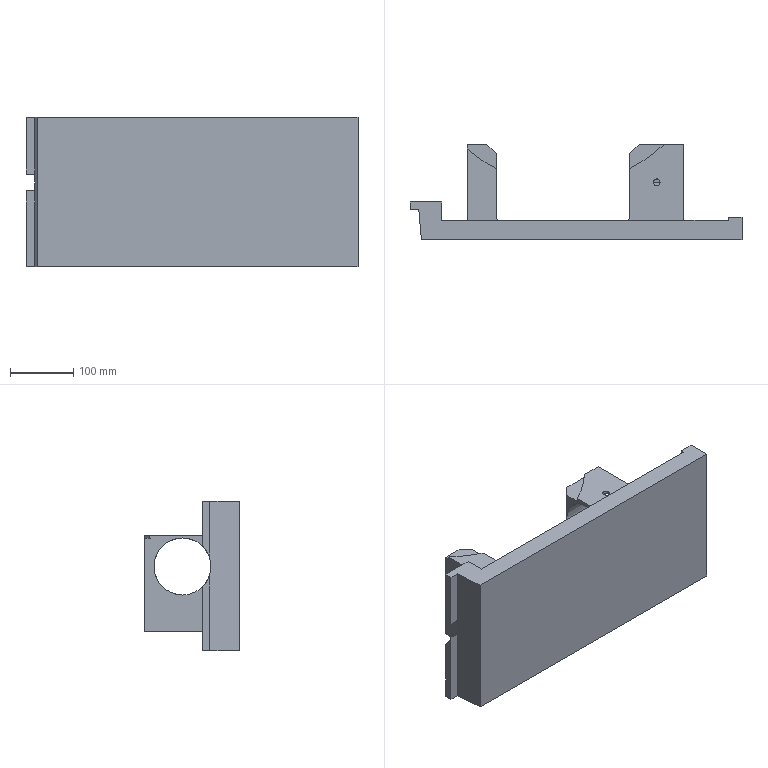Part | SolidWorks | features Cut 3, ICE 2, Extrusion 1, Fillet 1, HoleWzd 1, RevCut 1 | 1 solid | 48 faces | box 523 x 150 x 235 mm | volume 5356389 mm3 | plane 29 | cylinder 13 | cone 6 | commonest cylinder face diameters 90 x5 6.8 x4 10 x2 464 x2